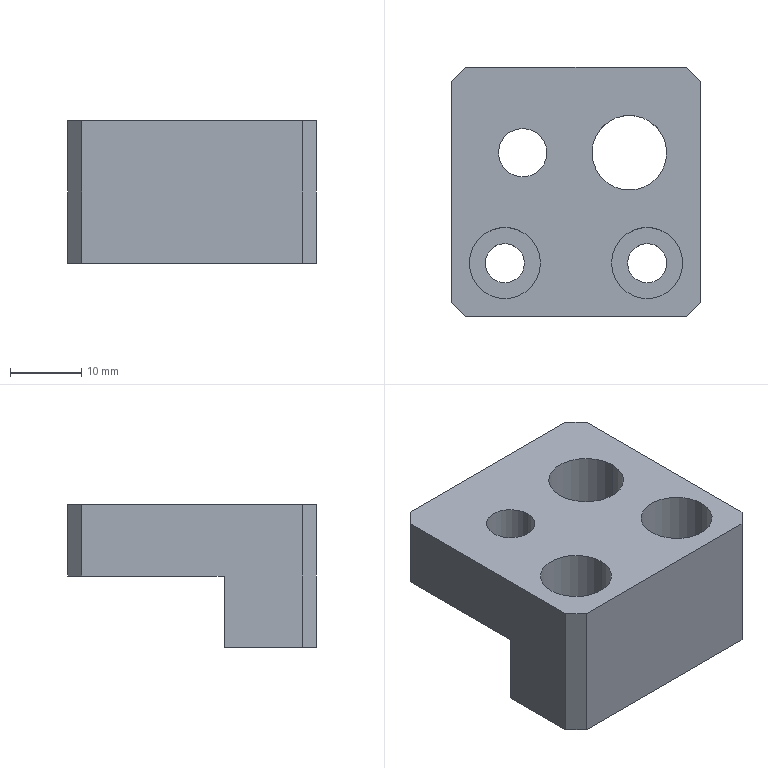Part | SolidWorks | features HoleWzd 3, Chamfer 1, Extrusion 1, ICE 1 | 1 solid | 26 faces | box 35 x 35 x 20 mm | volume 13186 mm3 | plane 14 | cylinder 12 | commonest cylinder face diameters 5.5 x4 10 x4 6.8 x2 10.5 x2
STEP:
#1=CARTESIAN_POINT('',(-15.,-10.,8.));
#2=VERTEX_POINT('',#1);
#3=CARTESIAN_POINT('',(-5.,-10.,8.));
#4=VERTEX_POINT('',#3);
#5=CARTESIAN_POINT('',(-10.,-10.,8.));
#6=DIRECTION('',(0.,0.,1.));
#7=DIRECTION('',(1.,0.,0.));
#8=AXIS2_PLACEMENT_3D('',#5,#6,#7);
#9=CIRCLE('',#8,5.);
#10=EDGE_CURVE('',#2,#4,#9,.T.);
#11=ORIENTED_EDGE('',*,*,#10,.F.);
#12=CARTESIAN_POINT('',(-15.,-10.,20.));
#13=VERTEX_POINT('',#12);
#14=CARTESIAN_POINT('',(-15.,-10.,20.));
#15=DIRECTION('',(0.,0.,1.));
#16=VECTOR('',#15,1000.);
#17=LINE('',#14,#16);
#18=EDGE_CURVE('',#2,#13,#17,.T.);
#19=ORIENTED_EDGE('',*,*,#18,.T.);
#20=CARTESIAN_POINT('',(-5.,-10.,20.));
#21=VERTEX_POINT('',#20);
#22=CARTESIAN_POINT('',(-10.,-10.,20.));
#23=DIRECTION('',(0.,0.,1.));
#24=DIRECTION('',(1.,0.,0.));
#25=AXIS2_PLACEMENT_3D('',#22,#23,#24);
#26=CIRCLE('',#25,5.);
#27=EDGE_CURVE('',#13,#21,#26,.T.);
#28=ORIENTED_EDGE('',*,*,#27,.T.);
#29=CARTESIAN_POINT('',(-5.,-10.,20.));
#30=DIRECTION('',(0.,0.,1.));
#31=VECTOR('',#30,1000.);
#32=LINE('',#29,#31);
#33=EDGE_CURVE('',#4,#21,#32,.T.);
#34=ORIENTED_EDGE('',*,*,#33,.F.);
#35=EDGE_LOOP('',(#11,#19,#28,#34));
#36=FACE_OUTER_BOUND('',#35,.T.);
#37=CARTESIAN_POINT('',(-10.,-10.,20.));
#38=DIRECTION('',(0.,0.,1.));
#39=DIRECTION('',(1.,0.,0.));
#40=AXIS2_PLACEMENT_3D('',#37,#38,#39);
#41=CYLINDRICAL_SURFACE('',#40,5.);
#42=ADVANCED_FACE('',(#36),#41,.F.);
#43=CARTESIAN_POINT('',(-12.75,-10.,0.));
#44=VERTEX_POINT('',#43);
#45=CARTESIAN_POINT('',(-7.25,-10.,0.));
#46=VERTEX_POINT('',#45);
#47=CARTESIAN_POINT('',(-10.,-10.,0.));
#48=DIRECTION('',(0.,0.,1.));
#49=DIRECTION('',(1.,0.,0.));
#50=AXIS2_PLACEMENT_3D('',#47,#48,#49);
#51=CIRCLE('',#50,2.75);
#52=EDGE_CURVE('',#44,#46,#51,.T.);
#53=ORIENTED_EDGE('',*,*,#52,.F.);
#54=CARTESIAN_POINT('',(-12.75,-10.,8.));
#55=VERTEX_POINT('',#54);
#56=CARTESIAN_POINT('',(-12.75,-10.,20.));
#57=DIRECTION('',(0.,0.,1.));
#58=VECTOR('',#57,1000.);
#59=LINE('',#56,#58);
#60=EDGE_CURVE('',#44,#55,#59,.T.);
#61=ORIENTED_EDGE('',*,*,#60,.T.);
#62=CARTESIAN_POINT('',(-7.25,-10.,8.));
#63=VERTEX_POINT('',#62);
#64=CARTESIAN_POINT('',(-10.,-10.,8.));
#65=DIRECTION('',(0.,0.,1.));
#66=DIRECTION('',(1.,0.,0.));
#67=AXIS2_PLACEMENT_3D('',#64,#65,#66);
#68=CIRCLE('',#67,2.75);
#69=EDGE_CURVE('',#55,#63,#68,.T.);
#70=ORIENTED_EDGE('',*,*,#69,.T.);
#71=CARTESIAN_POINT('',(-7.25,-10.,20.));
#72=DIRECTION('',(0.,0.,1.));
#73=VECTOR('',#72,1000.);
#74=LINE('',#71,#73);
#75=EDGE_CURVE('',#46,#63,#74,.T.);
#76=ORIENTED_EDGE('',*,*,#75,.F.);
#77=EDGE_LOOP('',(#53,#61,#70,#76));
#78=FACE_OUTER_BOUND('',#77,.T.);
#79=CARTESIAN_POINT('',(-10.,-10.,20.));
#80=DIRECTION('',(0.,0.,1.));
#81=DIRECTION('',(1.,0.,0.));
#82=AXIS2_PLACEMENT_3D('',#79,#80,#81);
#83=CYLINDRICAL_SURFACE('',#82,2.75);
#84=ADVANCED_FACE('',(#78),#83,.F.);
#85=CARTESIAN_POINT('',(5.,-10.,8.));
#86=VERTEX_POINT('',#85);
#87=CARTESIAN_POINT('',(15.,-10.,8.));
#88=VERTEX_POINT('',#87);
#89=CARTESIAN_POINT('',(10.,-10.,8.));
#90=DIRECTION('',(0.,0.,1.));
#91=DIRECTION('',(1.,0.,0.));
#92=AXIS2_PLACEMENT_3D('',#89,#90,#91);
#93=CIRCLE('',#92,5.);
#94=EDGE_CURVE('',#86,#88,#93,.T.);
#95=ORIENTED_EDGE('',*,*,#94,.F.);
#96=CARTESIAN_POINT('',(5.,-10.,20.));
#97=VERTEX_POINT('',#96);
#98=CARTESIAN_POINT('',(5.,-10.,20.));
#99=DIRECTION('',(0.,0.,1.));
#100=VECTOR('',#99,1000.);
#101=LINE('',#98,#100);
#102=EDGE_CURVE('',#86,#97,#101,.T.);
#103=ORIENTED_EDGE('',*,*,#102,.T.);
#104=CARTESIAN_POINT('',(15.,-10.,20.));
#105=VERTEX_POINT('',#104);
#106=CARTESIAN_POINT('',(10.,-10.,20.));
#107=DIRECTION('',(0.,0.,1.));
#108=DIRECTION('',(1.,0.,0.));
#109=AXIS2_PLACEMENT_3D('',#106,#107,#108);
#110=CIRCLE('',#109,5.);
#111=EDGE_CURVE('',#97,#105,#110,.T.);
#112=ORIENTED_EDGE('',*,*,#111,.T.);
#113=CARTESIAN_POINT('',(15.,-10.,20.));
#114=DIRECTION('',(0.,0.,1.));
#115=VECTOR('',#114,1000.);
#116=LINE('',#113,#115);
#117=EDGE_CURVE('',#88,#105,#116,.T.);
#118=ORIENTED_EDGE('',*,*,#117,.F.);
#119=EDGE_LOOP('',(#95,#103,#112,#118));
#120=FACE_OUTER_BOUND('',#119,.T.);
#121=CARTESIAN_POINT('',(10.,-10.,20.));
#122=DIRECTION('',(0.,0.,1.));
#123=DIRECTION('',(1.,0.,0.));
#124=AXIS2_PLACEMENT_3D('',#121,#122,#123);
#125=CYLINDRICAL_SURFACE('',#124,5.);
#126=ADVANCED_FACE('',(#120),#125,.F.);
#127=CARTESIAN_POINT('',(7.25,-10.,0.));
#128=VERTEX_POINT('',#127);
#129=CARTESIAN_POINT('',(12.75,-10.,0.));
#130=VERTEX_POINT('',#129);
#131=CARTESIAN_POINT('',(10.,-10.,0.));
#132=DIRECTION('',(0.,0.,1.));
#133=DIRECTION('',(1.,0.,0.));
#134=AXIS2_PLACEMENT_3D('',#131,#132,#133);
#135=CIRCLE('',#134,2.75);
#136=EDGE_CURVE('',#128,#130,#135,.T.);
#137=ORIENTED_EDGE('',*,*,#136,.F.);
#138=CARTESIAN_POINT('',(7.25,-10.,8.));
#139=VERTEX_POINT('',#138);
#140=CARTESIAN_POINT('',(7.25,-10.,20.));
#141=DIRECTION('',(0.,0.,1.));
#142=VECTOR('',#141,1000.);
#143=LINE('',#140,#142);
#144=EDGE_CURVE('',#128,#139,#143,.T.);
#145=ORIENTED_EDGE('',*,*,#144,.T.);
#146=CARTESIAN_POINT('',(12.75,-10.,8.));
#147=VERTEX_POINT('',#146);
#148=CARTESIAN_POINT('',(10.,-10.,8.));
#149=DIRECTION('',(0.,0.,1.));
#150=DIRECTION('',(1.,0.,0.));
#151=AXIS2_PLACEMENT_3D('',#148,#149,#150);
#152=CIRCLE('',#151,2.75);
#153=EDGE_CURVE('',#139,#147,#152,.T.);
#154=ORIENTED_EDGE('',*,*,#153,.T.);
#155=CARTESIAN_POINT('',(12.75,-10.,20.));
#156=DIRECTION('',(0.,0.,1.));
#157=VECTOR('',#156,1000.);
#158=LINE('',#155,#157);
#159=EDGE_CURVE('',#130,#147,#158,.T.);
#160=ORIENTED_EDGE('',*,*,#159,.F.);
#161=EDGE_LOOP('',(#137,#145,#154,#160));
#162=FACE_OUTER_BOUND('',#161,.T.);
#163=CARTESIAN_POINT('',(10.,-10.,20.));
#164=DIRECTION('',(0.,0.,1.));
#165=DIRECTION('',(1.,0.,0.));
#166=AXIS2_PLACEMENT_3D('',#163,#164,#165);
#167=CYLINDRICAL_SURFACE('',#166,2.75);
#168=ADVANCED_FACE('',(#162),#167,.F.);
#169=CARTESIAN_POINT('',(-4.1,5.5,10.));
#170=VERTEX_POINT('',#169);
#171=CARTESIAN_POINT('',(-10.9,5.5,10.));
#172=VERTEX_POINT('',#171);
#173=CARTESIAN_POINT('',(-7.5,5.5,10.));
#174=DIRECTION('',(0.,0.,-1.));
#175=DIRECTION('',(0.,-1.,0.));
#176=AXIS2_PLACEMENT_3D('',#173,#174,#175);
#177=CIRCLE('',#176,3.4);
#178=EDGE_CURVE('',#170,#172,#177,.T.);
#179=ORIENTED_EDGE('',*,*,#178,.T.);
#180=CARTESIAN_POINT('',(-10.9,5.5,20.));
#181=VERTEX_POINT('',#180);
#182=CARTESIAN_POINT('',(-10.9,5.5,20.));
#183=DIRECTION('',(0.,0.,1.));
#184=VECTOR('',#183,1000.);
#185=LINE('',#182,#184);
#186=EDGE_CURVE('',#172,#181,#185,.T.);
#187=ORIENTED_EDGE('',*,*,#186,.T.);
#188=CARTESIAN_POINT('',(-4.1,5.5,20.));
#189=VERTEX_POINT('',#188);
#190=CARTESIAN_POINT('',(-7.5,5.5,20.));
#191=DIRECTION('',(0.,0.,1.));
#192=DIRECTION('',(1.,0.,0.));
#193=AXIS2_PLACEMENT_3D('',#190,#191,#192);
#194=CIRCLE('',#193,3.4);
#195=EDGE_CURVE('',#181,#189,#194,.T.);
#196=ORIENTED_EDGE('',*,*,#195,.T.);
#197=CARTESIAN_POINT('',(-4.1,5.5,20.));
#198=DIRECTION('',(0.,0.,1.));
#199=VECTOR('',#198,1000.);
#200=LINE('',#197,#199);
#201=EDGE_CURVE('',#170,#189,#200,.T.);
#202=ORIENTED_EDGE('',*,*,#201,.F.);
#203=EDGE_LOOP('',(#179,#187,#196,#202));
#204=FACE_OUTER_BOUND('',#203,.T.);
#205=CARTESIAN_POINT('',(-7.5,5.5,20.));
#206=DIRECTION('',(0.,0.,1.));
#207=DIRECTION('',(1.,0.,0.));
#208=AXIS2_PLACEMENT_3D('',#205,#206,#207);
#209=CYLINDRICAL_SURFACE('',#208,3.4);
#210=ADVANCED_FACE('',(#204),#209,.F.);
#211=CARTESIAN_POINT('',(12.75,5.5,10.));
#212=VERTEX_POINT('',#211);
#213=CARTESIAN_POINT('',(2.25,5.5,10.));
#214=VERTEX_POINT('',#213);
#215=CARTESIAN_POINT('',(7.5,5.5,10.));
#216=DIRECTION('',(0.,0.,-1.));
#217=DIRECTION('',(0.,-1.,0.));
#218=AXIS2_PLACEMENT_3D('',#215,#216,#217);
#219=CIRCLE('',#218,5.25);
#220=EDGE_CURVE('',#212,#214,#219,.T.);
#221=ORIENTED_EDGE('',*,*,#220,.T.);
#222=CARTESIAN_POINT('',(2.25,5.5,20.));
#223=VERTEX_POINT('',#222);
#224=CARTESIAN_POINT('',(2.25,5.5,20.));
#225=DIRECTION('',(0.,0.,1.));
#226=VECTOR('',#225,1000.);
#227=LINE('',#224,#226);
#228=EDGE_CURVE('',#214,#223,#227,.T.);
#229=ORIENTED_EDGE('',*,*,#228,.T.);
#230=CARTESIAN_POINT('',(12.75,5.5,20.));
#231=VERTEX_POINT('',#230);
#232=CARTESIAN_POINT('',(7.5,5.5,20.));
#233=DIRECTION('',(0.,0.,1.));
#234=DIRECTION('',(1.,0.,0.));
#235=AXIS2_PLACEMENT_3D('',#232,#233,#234);
#236=CIRCLE('',#235,5.25);
#237=EDGE_CURVE('',#223,#231,#236,.T.);
#238=ORIENTED_EDGE('',*,*,#237,.T.);
#239=CARTESIAN_POINT('',(12.75,5.5,20.));
#240=DIRECTION('',(0.,0.,1.));
#241=VECTOR('',#240,1000.);
#242=LINE('',#239,#241);
#243=EDGE_CURVE('',#212,#231,#242,.T.);
#244=ORIENTED_EDGE('',*,*,#243,.F.);
#245=EDGE_LOOP('',(#221,#229,#238,#244));
#246=FACE_OUTER_BOUND('',#245,.T.);
#247=CARTESIAN_POINT('',(7.5,5.5,20.));
#248=DIRECTION('',(0.,0.,1.));
#249=DIRECTION('',(1.,0.,0.));
#250=AXIS2_PLACEMENT_3D('',#247,#248,#249);
#251=CYLINDRICAL_SURFACE('',#250,5.25);
#252=ADVANCED_FACE('',(#246),#251,.F.);
#253=CARTESIAN_POINT('',(17.5,-15.5,0.));
#254=VERTEX_POINT('',#253);
#255=CARTESIAN_POINT('',(17.5,-4.5,0.));
#256=VERTEX_POINT('',#255);
#257=CARTESIAN_POINT('',(17.5,-17.5,0.));
#258=DIRECTION('',(0.,1.,0.));
#259=VECTOR('',#258,1000.);
#260=LINE('',#257,#259);
#261=EDGE_CURVE('',#254,#256,#260,.T.);
#262=ORIENTED_EDGE('',*,*,#261,.T.);
#263=CARTESIAN_POINT('',(17.5,-4.5,10.));
#264=VERTEX_POINT('',#263);
#265=CARTESIAN_POINT('',(17.5,-4.5,0.));
#266=DIRECTION('',(0.,0.,-1.));
#267=VECTOR('',#266,1000.);
#268=LINE('',#265,#267);
#269=EDGE_CURVE('',#264,#256,#268,.T.);
#270=ORIENTED_EDGE('',*,*,#269,.F.);
#271=CARTESIAN_POINT('',(17.5,15.5,10.));
#272=VERTEX_POINT('',#271);
#273=CARTESIAN_POINT('',(17.5,17.5,10.));
#274=DIRECTION('',(0.,-1.,0.));
#275=VECTOR('',#274,1000.);
#276=LINE('',#273,#275);
#277=EDGE_CURVE('',#272,#264,#276,.T.);
#278=ORIENTED_EDGE('',*,*,#277,.F.);
#279=CARTESIAN_POINT('',(17.5,15.5,20.));
#280=VERTEX_POINT('',#279);
#281=CARTESIAN_POINT('',(17.5,15.5,20.));
#282=DIRECTION('',(0.,0.,1.));
#283=VECTOR('',#282,1000.);
#284=LINE('',#281,#283);
#285=EDGE_CURVE('',#272,#280,#284,.T.);
#286=ORIENTED_EDGE('',*,*,#285,.T.);
#287=CARTESIAN_POINT('',(17.5,-15.5,20.));
#288=VERTEX_POINT('',#287);
#289=CARTESIAN_POINT('',(17.5,-17.5,20.));
#290=DIRECTION('',(0.,1.,0.));
#291=VECTOR('',#290,1000.);
#292=LINE('',#289,#291);
#293=EDGE_CURVE('',#288,#280,#292,.T.);
#294=ORIENTED_EDGE('',*,*,#293,.F.);
#295=CARTESIAN_POINT('',(17.5,-15.5,20.));
#296=DIRECTION('',(0.,0.,-1.));
#297=VECTOR('',#296,1000.);
#298=LINE('',#295,#297);
#299=EDGE_CURVE('',#288,#254,#298,.T.);
#300=ORIENTED_EDGE('',*,*,#299,.T.);
#301=EDGE_LOOP('',(#262,#270,#278,#286,#294,#300));
#302=FACE_OUTER_BOUND('',#301,.T.);
#303=CARTESIAN_POINT('',(17.5,-17.5,20.));
#304=DIRECTION('',(-1.,0.,0.));
#305=DIRECTION('',(0.,0.,1.));
#306=AXIS2_PLACEMENT_3D('',#303,#304,#305);
#307=PLANE('',#306);
#308=ADVANCED_FACE('',(#302),#307,.F.);
#309=CARTESIAN_POINT('',(15.5,17.5,20.));
#310=VERTEX_POINT('',#309);
#311=CARTESIAN_POINT('',(15.5,17.5,10.));
#312=VERTEX_POINT('',#311);
#313=CARTESIAN_POINT('',(15.5,17.5,20.));
#314=DIRECTION('',(0.,0.,-1.));
#315=VECTOR('',#314,1000.);
#316=LINE('',#313,#315);
#317=EDGE_CURVE('',#310,#312,#316,.T.);
#318=ORIENTED_EDGE('',*,*,#317,.T.);
#319=CARTESIAN_POINT('',(-15.5,17.5,10.));
#320=VERTEX_POINT('',#319);
#321=CARTESIAN_POINT('',(-17.5,17.5,10.));
#322=DIRECTION('',(1.,0.,0.));
#323=VECTOR('',#322,1000.);
#324=LINE('',#321,#323);
#325=EDGE_CURVE('',#320,#312,#324,.T.);
#326=ORIENTED_EDGE('',*,*,#325,.F.);
#327=CARTESIAN_POINT('',(-15.5,17.5,20.));
#328=VERTEX_POINT('',#327);
#329=CARTESIAN_POINT('',(-15.5,17.5,20.));
#330=DIRECTION('',(0.,0.,1.));
#331=VECTOR('',#330,1000.);
#332=LINE('',#329,#331);
#333=EDGE_CURVE('',#320,#328,#332,.T.);
#334=ORIENTED_EDGE('',*,*,#333,.T.);
#335=CARTESIAN_POINT('',(-17.5,17.5,20.));
#336=DIRECTION('',(-1.,0.,0.));
#337=VECTOR('',#336,1000.);
#338=LINE('',#335,#337);
#339=EDGE_CURVE('',#310,#328,#338,.T.);
#340=ORIENTED_EDGE('',*,*,#339,.F.);
#341=EDGE_LOOP('',(#318,#326,#334,#340));
#342=FACE_OUTER_BOUND('',#341,.T.);
#343=CARTESIAN_POINT('',(-17.5,17.5,20.));
#344=DIRECTION('',(0.,-1.,0.));
#345=DIRECTION('',(0.,0.,-1.));
#346=AXIS2_PLACEMENT_3D('',#343,#344,#345);
#347=PLANE('',#346);
#348=ADVANCED_FACE('',(#342),#347,.F.);
#349=CARTESIAN_POINT('',(-17.5,15.5,10.));
#350=VERTEX_POINT('',#349);
#351=CARTESIAN_POINT('',(-17.5,-4.5,10.));
#352=VERTEX_POINT('',#351);
#353=CARTESIAN_POINT('',(-17.5,17.5,10.));
#354=DIRECTION('',(0.,-1.,0.));
#355=VECTOR('',#354,1000.);
#356=LINE('',#353,#355);
#357=EDGE_CURVE('',#350,#352,#356,.T.);
#358=ORIENTED_EDGE('',*,*,#357,.T.);
#359=CARTESIAN_POINT('',(-17.5,-4.5,0.));
#360=VERTEX_POINT('',#359);
#361=CARTESIAN_POINT('',(-17.5,-4.5,0.));
#362=DIRECTION('',(0.,0.,-1.));
#363=VECTOR('',#362,1000.);
#364=LINE('',#361,#363);
#365=EDGE_CURVE('',#352,#360,#364,.T.);
#366=ORIENTED_EDGE('',*,*,#365,.T.);
#367=CARTESIAN_POINT('',(-17.5,-15.5,0.));
#368=VERTEX_POINT('',#367);
#369=CARTESIAN_POINT('',(-17.5,-17.5,0.));
#370=DIRECTION('',(0.,-1.,0.));
#371=VECTOR('',#370,1000.);
#372=LINE('',#369,#371);
#373=EDGE_CURVE('',#360,#368,#372,.T.);
#374=ORIENTED_EDGE('',*,*,#373,.T.);
#375=CARTESIAN_POINT('',(-17.5,-15.5,20.));
#376=VERTEX_POINT('',#375);
#377=CARTESIAN_POINT('',(-17.5,-15.5,20.));
#378=DIRECTION('',(0.,0.,1.));
#379=VECTOR('',#378,1000.);
#380=LINE('',#377,#379);
#381=EDGE_CURVE('',#368,#376,#380,.T.);
#382=ORIENTED_EDGE('',*,*,#381,.T.);
#383=CARTESIAN_POINT('',(-17.5,15.5,20.));
#384=VERTEX_POINT('',#383);
#385=CARTESIAN_POINT('',(-17.5,-17.5,20.));
#386=DIRECTION('',(0.,-1.,0.));
#387=VECTOR('',#386,1000.);
#388=LINE('',#385,#387);
#389=EDGE_CURVE('',#384,#376,#388,.T.);
#390=ORIENTED_EDGE('',*,*,#389,.F.);
#391=CARTESIAN_POINT('',(-17.5,15.5,20.));
#392=DIRECTION('',(0.,0.,-1.));
#393=VECTOR('',#392,1000.);
#394=LINE('',#391,#393);
#395=EDGE_CURVE('',#384,#350,#394,.T.);
#396=ORIENTED_EDGE('',*,*,#395,.T.);
#397=EDGE_LOOP('',(#358,#366,#374,#382,#390,#396));
#398=FACE_OUTER_BOUND('',#397,.T.);
#399=CARTESIAN_POINT('',(-17.5,-17.5,20.));
#400=DIRECTION('',(1.,0.,0.));
#401=DIRECTION('',(0.,0.,-1.));
#402=AXIS2_PLACEMENT_3D('',#399,#400,#401);
#403=PLANE('',#402);
#404=ADVANCED_FACE('',(#398),#403,.F.);
#405=CARTESIAN_POINT('',(-15.5,-17.5,0.));
#406=VERTEX_POINT('',#405);
#407=CARTESIAN_POINT('',(15.5,-17.5,0.));
#408=VERTEX_POINT('',#407);
#409=CARTESIAN_POINT('',(-17.5,-17.5,0.));
#410=DIRECTION('',(1.,0.,0.));
#411=VECTOR('',#410,1000.);
#412=LINE('',#409,#411);
#413=EDGE_CURVE('',#406,#408,#412,.T.);
#414=ORIENTED_EDGE('',*,*,#413,.T.);
#415=CARTESIAN_POINT('',(15.5,-17.5,20.));
#416=VERTEX_POINT('',#415);
#417=CARTESIAN_POINT('',(15.5,-17.5,20.));
#418=DIRECTION('',(0.,0.,1.));
#419=VECTOR('',#418,1000.);
#420=LINE('',#417,#419);
#421=EDGE_CURVE('',#408,#416,#420,.T.);
#422=ORIENTED_EDGE('',*,*,#421,.T.);
#423=CARTESIAN_POINT('',(-15.5,-17.5,20.));
#424=VERTEX_POINT('',#423);
#425=CARTESIAN_POINT('',(-17.5,-17.5,20.));
#426=DIRECTION('',(1.,0.,0.));
#427=VECTOR('',#426,1000.);
#428=LINE('',#425,#427);
#429=EDGE_CURVE('',#424,#416,#428,.T.);
#430=ORIENTED_EDGE('',*,*,#429,.F.);
#431=CARTESIAN_POINT('',(-15.5,-17.5,20.));
#432=DIRECTION('',(0.,0.,-1.));
#433=VECTOR('',#432,1000.);
#434=LINE('',#431,#433);
#435=EDGE_CURVE('',#424,#406,#434,.T.);
#436=ORIENTED_EDGE('',*,*,#435,.T.);
#437=EDGE_LOOP('',(#414,#422,#430,#436));
#438=FACE_OUTER_BOUND('',#437,.T.);
#439=CARTESIAN_POINT('',(-17.5,-17.5,20.));
#440=DIRECTION('',(0.,1.,0.));
#441=DIRECTION('',(0.,0.,1.));
#442=AXIS2_PLACEMENT_3D('',#439,#440,#441);
#443=PLANE('',#442);
#444=ADVANCED_FACE('',(#438),#443,.F.);
#445=CARTESIAN_POINT('',(-10.,-10.,20.));
#446=DIRECTION('',(0.,0.,1.));
#447=DIRECTION('',(1.,0.,0.));
#448=AXIS2_PLACEMENT_3D('',#445,#446,#447);
#449=CIRCLE('',#448,5.);
#450=EDGE_CURVE('',#21,#13,#449,.T.);
#451=ORIENTED_EDGE('',*,*,#450,.F.);
#452=ORIENTED_EDGE('',*,*,#27,.F.);
#453=EDGE_LOOP('',(#451,#452));
#454=FACE_BOUND('',#453,.T.);
#455=CARTESIAN_POINT('',(10.,-10.,20.));
#456=DIRECTION('',(0.,0.,1.));
#457=DIRECTION('',(1.,0.,0.));
#458=AXIS2_PLACEMENT_3D('',#455,#456,#457);
#459=CIRCLE('',#458,5.);
#460=EDGE_CURVE('',#105,#97,#459,.T.);
#461=ORIENTED_EDGE('',*,*,#460,.F.);
#462=ORIENTED_EDGE('',*,*,#111,.F.);
#463=EDGE_LOOP('',(#461,#462));
#464=FACE_BOUND('',#463,.T.);
#465=CARTESIAN_POINT('',(-7.5,5.5,20.));
#466=DIRECTION('',(0.,0.,1.));
#467=DIRECTION('',(1.,0.,0.));
#468=AXIS2_PLACEMENT_3D('',#465,#466,#467);
#469=CIRCLE('',#468,3.4);
#470=EDGE_CURVE('',#189,#181,#469,.T.);
#471=ORIENTED_EDGE('',*,*,#470,.F.);
#472=ORIENTED_EDGE('',*,*,#195,.F.);
#473=EDGE_LOOP('',(#471,#472));
#474=FACE_BOUND('',#473,.T.);
#475=CARTESIAN_POINT('',(7.5,5.5,20.));
#476=DIRECTION('',(0.,0.,1.));
#477=DIRECTION('',(1.,0.,0.));
#478=AXIS2_PLACEMENT_3D('',#475,#476,#477);
#479=CIRCLE('',#478,5.25);
#480=EDGE_CURVE('',#231,#223,#479,.T.);
#481=ORIENTED_EDGE('',*,*,#480,.F.);
#482=ORIENTED_EDGE('',*,*,#237,.F.);
#483=EDGE_LOOP('',(#481,#482));
#484=FACE_BOUND('',#483,.T.);
#485=ORIENTED_EDGE('',*,*,#429,.T.);
#486=CARTESIAN_POINT('',(17.5,-15.5,20.));
#487=DIRECTION('',(0.7071,0.7071,0.));
#488=VECTOR('',#487,1000.);
#489=LINE('',#486,#488);
#490=EDGE_CURVE('',#416,#288,#489,.T.);
#491=ORIENTED_EDGE('',*,*,#490,.T.);
#492=ORIENTED_EDGE('',*,*,#293,.T.);
#493=CARTESIAN_POINT('',(15.5,17.5,20.));
#494=DIRECTION('',(-0.7071,0.7071,0.));
#495=VECTOR('',#494,1000.);
#496=LINE('',#493,#495);
#497=EDGE_CURVE('',#280,#310,#496,.T.);
#498=ORIENTED_EDGE('',*,*,#497,.T.);
#499=ORIENTED_EDGE('',*,*,#339,.T.);
#500=CARTESIAN_POINT('',(-17.5,15.5,20.));
#501=DIRECTION('',(-0.7071,-0.7071,0.));
#502=VECTOR('',#501,1000.);
#503=LINE('',#500,#502);
#504=EDGE_CURVE('',#328,#384,#503,.T.);
#505=ORIENTED_EDGE('',*,*,#504,.T.);
#506=ORIENTED_EDGE('',*,*,#389,.T.);
#507=CARTESIAN_POINT('',(-15.5,-17.5,20.));
#508=DIRECTION('',(0.7071,-0.7071,0.));
#509=VECTOR('',#508,1000.);
#510=LINE('',#507,#509);
#511=EDGE_CURVE('',#376,#424,#510,.T.);
#512=ORIENTED_EDGE('',*,*,#511,.T.);
#513=EDGE_LOOP('',(#485,#491,#492,#498,#499,#505,#506,#512));
#514=FACE_OUTER_BOUND('',#513,.T.);
#515=CARTESIAN_POINT('',(0.,0.,20.));
#516=DIRECTION('',(0.,0.,-1.));
#517=DIRECTION('',(-1.,0.,0.));
#518=AXIS2_PLACEMENT_3D('',#515,#516,#517);
#519=PLANE('',#518);
#520=ADVANCED_FACE('',(#454,#464,#474,#484,#514),#519,.F.);
#521=CARTESIAN_POINT('',(-17.5,-4.5,0.));
#522=DIRECTION('',(1.,0.,0.));
#523=VECTOR('',#522,1000.);
#524=LINE('',#521,#523);
#525=EDGE_CURVE('',#360,#256,#524,.T.);
#526=ORIENTED_EDGE('',*,*,#525,.T.);
#527=ORIENTED_EDGE('',*,*,#261,.F.);
#528=CARTESIAN_POINT('',(16.5,-16.5,0.));
#529=DIRECTION('',(-0.7071,-0.7071,0.));
#530=VECTOR('',#529,1000.);
#531=LINE('',#528,#530);
#532=EDGE_CURVE('',#254,#408,#531,.T.);
#533=ORIENTED_EDGE('',*,*,#532,.T.);
#534=ORIENTED_EDGE('',*,*,#413,.F.);
#535=CARTESIAN_POINT('',(-16.5,-16.5,0.));
#536=DIRECTION('',(-0.7071,0.7071,0.));
#537=VECTOR('',#536,1000.);
#538=LINE('',#535,#537);
#539=EDGE_CURVE('',#406,#368,#538,.T.);
#540=ORIENTED_EDGE('',*,*,#539,.T.);
#541=ORIENTED_EDGE('',*,*,#373,.F.);
#542=EDGE_LOOP('',(#526,#527,#533,#534,#540,#541));
#543=FACE_OUTER_BOUND('',#542,.T.);
#544=CARTESIAN_POINT('',(-10.,-10.,0.));
#545=DIRECTION('',(0.,0.,1.));
#546=DIRECTION('',(1.,0.,0.));
#547=AXIS2_PLACEMENT_3D('',#544,#545,#546);
#548=CIRCLE('',#547,2.75);
#549=EDGE_CURVE('',#46,#44,#548,.T.);
#550=ORIENTED_EDGE('',*,*,#549,.T.);
#551=ORIENTED_EDGE('',*,*,#52,.T.);
#552=EDGE_LOOP('',(#550,#551));
#553=FACE_BOUND('',#552,.T.);
#554=CARTESIAN_POINT('',(10.,-10.,0.));
#555=DIRECTION('',(0.,0.,1.));
#556=DIRECTION('',(1.,0.,0.));
#557=AXIS2_PLACEMENT_3D('',#554,#555,#556);
#558=CIRCLE('',#557,2.75);
#559=EDGE_CURVE('',#130,#128,#558,.T.);
#560=ORIENTED_EDGE('',*,*,#559,.T.);
#561=ORIENTED_EDGE('',*,*,#136,.T.);
#562=EDGE_LOOP('',(#560,#561));
#563=FACE_BOUND('',#562,.T.);
#564=CARTESIAN_POINT('',(0.,0.,0.));
#565=DIRECTION('',(0.,0.,-1.));
#566=DIRECTION('',(-1.,0.,0.));
#567=AXIS2_PLACEMENT_3D('',#564,#565,#566);
#568=PLANE('',#567);
#569=ADVANCED_FACE('',(#543,#553,#563),#568,.T.);
#570=ORIENTED_EDGE('',*,*,#490,.F.);
#571=ORIENTED_EDGE('',*,*,#421,.F.);
#572=ORIENTED_EDGE('',*,*,#532,.F.);
#573=ORIENTED_EDGE('',*,*,#299,.F.);
#574=EDGE_LOOP('',(#570,#571,#572,#573));
#575=FACE_OUTER_BOUND('',#574,.T.);
#576=CARTESIAN_POINT('',(17.5,-15.5,20.));
#577=DIRECTION('',(-0.7071,0.7071,0.));
#578=DIRECTION('',(0.,0.,-1.));
#579=AXIS2_PLACEMENT_3D('',#576,#577,#578);
#580=PLANE('',#579);
#581=ADVANCED_FACE('',(#575),#580,.F.);
#582=ORIENTED_EDGE('',*,*,#511,.F.);
#583=ORIENTED_EDGE('',*,*,#381,.F.);
#584=ORIENTED_EDGE('',*,*,#539,.F.);
#585=ORIENTED_EDGE('',*,*,#435,.F.);
#586=EDGE_LOOP('',(#582,#583,#584,#585));
#587=FACE_OUTER_BOUND('',#586,.T.);
#588=CARTESIAN_POINT('',(-15.5,-17.5,20.));
#589=DIRECTION('',(0.7071,0.7071,0.));
#590=DIRECTION('',(0.,0.,-1.));
#591=AXIS2_PLACEMENT_3D('',#588,#589,#590);
#592=PLANE('',#591);
#593=ADVANCED_FACE('',(#587),#592,.F.);
#594=CARTESIAN_POINT('',(-17.5,15.5,10.));
#595=DIRECTION('',(0.7071,0.7071,0.));
#596=VECTOR('',#595,1000.);
#597=LINE('',#594,#596);
#598=EDGE_CURVE('',#350,#320,#597,.T.);
#599=ORIENTED_EDGE('',*,*,#598,.F.);
#600=ORIENTED_EDGE('',*,*,#395,.F.);
#601=ORIENTED_EDGE('',*,*,#504,.F.);
#602=ORIENTED_EDGE('',*,*,#333,.F.);
#603=EDGE_LOOP('',(#599,#600,#601,#602));
#604=FACE_OUTER_BOUND('',#603,.T.);
#605=CARTESIAN_POINT('',(-17.5,15.5,20.));
#606=DIRECTION('',(0.7071,-0.7071,0.));
#607=DIRECTION('',(0.,0.,-1.));
#608=AXIS2_PLACEMENT_3D('',#605,#606,#607);
#609=PLANE('',#608);
#610=ADVANCED_FACE('',(#604),#609,.F.);
#611=CARTESIAN_POINT('',(15.5,17.5,10.));
#612=DIRECTION('',(0.7071,-0.7071,0.));
#613=VECTOR('',#612,1000.);
#614=LINE('',#611,#613);
#615=EDGE_CURVE('',#312,#272,#614,.T.);
#616=ORIENTED_EDGE('',*,*,#615,.F.);
#617=ORIENTED_EDGE('',*,*,#317,.F.);
#618=ORIENTED_EDGE('',*,*,#497,.F.);
#619=ORIENTED_EDGE('',*,*,#285,.F.);
#620=EDGE_LOOP('',(#616,#617,#618,#619));
#621=FACE_OUTER_BOUND('',#620,.T.);
#622=CARTESIAN_POINT('',(15.5,17.5,20.));
#623=DIRECTION('',(-0.7071,-0.7071,0.));
#624=DIRECTION('',(0.,0.,-1.));
#625=AXIS2_PLACEMENT_3D('',#622,#623,#624);
#626=PLANE('',#625);
#627=ADVANCED_FACE('',(#621),#626,.F.);
#628=ORIENTED_EDGE('',*,*,#228,.F.);
#629=CARTESIAN_POINT('',(7.5,5.5,10.));
#630=DIRECTION('',(0.,0.,-1.));
#631=DIRECTION('',(0.,-1.,0.));
#632=AXIS2_PLACEMENT_3D('',#629,#630,#631);
#633=CIRCLE('',#632,5.25);
#634=EDGE_CURVE('',#214,#212,#633,.T.);
#635=ORIENTED_EDGE('',*,*,#634,.T.);
#636=ORIENTED_EDGE('',*,*,#243,.T.);
#637=ORIENTED_EDGE('',*,*,#480,.T.);
#638=EDGE_LOOP('',(#628,#635,#636,#637));
#639=FACE_OUTER_BOUND('',#638,.T.);
#640=CARTESIAN_POINT('',(7.5,5.5,20.));
#641=DIRECTION('',(0.,0.,1.));
#642=DIRECTION('',(1.,0.,0.));
#643=AXIS2_PLACEMENT_3D('',#640,#641,#642);
#644=CYLINDRICAL_SURFACE('',#643,5.25);
#645=ADVANCED_FACE('',(#639),#644,.F.);
#646=ORIENTED_EDGE('',*,*,#186,.F.);
#647=CARTESIAN_POINT('',(-7.5,5.5,10.));
#648=DIRECTION('',(0.,0.,-1.));
#649=DIRECTION('',(0.,-1.,0.));
#650=AXIS2_PLACEMENT_3D('',#647,#648,#649);
#651=CIRCLE('',#650,3.4);
#652=EDGE_CURVE('',#172,#170,#651,.T.);
#653=ORIENTED_EDGE('',*,*,#652,.T.);
#654=ORIENTED_EDGE('',*,*,#201,.T.);
#655=ORIENTED_EDGE('',*,*,#470,.T.);
#656=EDGE_LOOP('',(#646,#653,#654,#655));
#657=FACE_OUTER_BOUND('',#656,.T.);
#658=CARTESIAN_POINT('',(-7.5,5.5,20.));
#659=DIRECTION('',(0.,0.,1.));
#660=DIRECTION('',(1.,0.,0.));
#661=AXIS2_PLACEMENT_3D('',#658,#659,#660);
#662=CYLINDRICAL_SURFACE('',#661,3.4);
#663=ADVANCED_FACE('',(#657),#662,.F.);
#664=ORIENTED_EDGE('',*,*,#144,.F.);
#665=ORIENTED_EDGE('',*,*,#559,.F.);
#666=ORIENTED_EDGE('',*,*,#159,.T.);
#667=CARTESIAN_POINT('',(10.,-10.,8.));
#668=DIRECTION('',(0.,0.,1.));
#669=DIRECTION('',(1.,0.,0.));
#670=AXIS2_PLACEMENT_3D('',#667,#668,#669);
#671=CIRCLE('',#670,2.75);
#672=EDGE_CURVE('',#147,#139,#671,.T.);
#673=ORIENTED_EDGE('',*,*,#672,.T.);
#674=EDGE_LOOP('',(#664,#665,#666,#673));
#675=FACE_OUTER_BOUND('',#674,.T.);
#676=CARTESIAN_POINT('',(10.,-10.,20.));
#677=DIRECTION('',(0.,0.,1.));
#678=DIRECTION('',(1.,0.,0.));
#679=AXIS2_PLACEMENT_3D('',#676,#677,#678);
#680=CYLINDRICAL_SURFACE('',#679,2.75);
#681=ADVANCED_FACE('',(#675),#680,.F.);
#682=ORIENTED_EDGE('',*,*,#672,.F.);
#683=ORIENTED_EDGE('',*,*,#153,.F.);
#684=EDGE_LOOP('',(#682,#683));
#685=FACE_BOUND('',#684,.T.);
#686=CARTESIAN_POINT('',(10.,-10.,8.));
#687=DIRECTION('',(0.,0.,1.));
#688=DIRECTION('',(1.,0.,0.));
#689=AXIS2_PLACEMENT_3D('',#686,#687,#688);
#690=CIRCLE('',#689,5.);
#691=EDGE_CURVE('',#88,#86,#690,.T.);
#692=ORIENTED_EDGE('',*,*,#691,.T.);
#693=ORIENTED_EDGE('',*,*,#94,.T.);
#694=EDGE_LOOP('',(#692,#693));
#695=FACE_OUTER_BOUND('',#694,.T.);
#696=CARTESIAN_POINT('',(12.75,-10.,8.));
#697=DIRECTION('',(0.,0.,-1.));
#698=DIRECTION('',(-1.,0.,0.));
#699=AXIS2_PLACEMENT_3D('',#696,#697,#698);
#700=PLANE('',#699);
#701=ADVANCED_FACE('',(#685,#695),#700,.F.);
#702=ORIENTED_EDGE('',*,*,#102,.F.);
#703=ORIENTED_EDGE('',*,*,#691,.F.);
#704=ORIENTED_EDGE('',*,*,#117,.T.);
#705=ORIENTED_EDGE('',*,*,#460,.T.);
#706=EDGE_LOOP('',(#702,#703,#704,#705));
#707=FACE_OUTER_BOUND('',#706,.T.);
#708=CARTESIAN_POINT('',(10.,-10.,20.));
#709=DIRECTION('',(0.,0.,1.));
#710=DIRECTION('',(1.,0.,0.));
#711=AXIS2_PLACEMENT_3D('',#708,#709,#710);
#712=CYLINDRICAL_SURFACE('',#711,5.);
#713=ADVANCED_FACE('',(#707),#712,.F.);
#714=ORIENTED_EDGE('',*,*,#60,.F.);
#715=ORIENTED_EDGE('',*,*,#549,.F.);
#716=ORIENTED_EDGE('',*,*,#75,.T.);
#717=CARTESIAN_POINT('',(-10.,-10.,8.));
#718=DIRECTION('',(0.,0.,1.));
#719=DIRECTION('',(1.,0.,0.));
#720=AXIS2_PLACEMENT_3D('',#717,#718,#719);
#721=CIRCLE('',#720,2.75);
#722=EDGE_CURVE('',#63,#55,#721,.T.);
#723=ORIENTED_EDGE('',*,*,#722,.T.);
#724=EDGE_LOOP('',(#714,#715,#716,#723));
#725=FACE_OUTER_BOUND('',#724,.T.);
#726=CARTESIAN_POINT('',(-10.,-10.,20.));
#727=DIRECTION('',(0.,0.,1.));
#728=DIRECTION('',(1.,0.,0.));
#729=AXIS2_PLACEMENT_3D('',#726,#727,#728);
#730=CYLINDRICAL_SURFACE('',#729,2.75);
#731=ADVANCED_FACE('',(#725),#730,.F.);
#732=ORIENTED_EDGE('',*,*,#722,.F.);
#733=ORIENTED_EDGE('',*,*,#69,.F.);
#734=EDGE_LOOP('',(#732,#733));
#735=FACE_BOUND('',#734,.T.);
#736=CARTESIAN_POINT('',(-10.,-10.,8.));
#737=DIRECTION('',(0.,0.,1.));
#738=DIRECTION('',(1.,0.,0.));
#739=AXIS2_PLACEMENT_3D('',#736,#737,#738);
#740=CIRCLE('',#739,5.);
#741=EDGE_CURVE('',#4,#2,#740,.T.);
#742=ORIENTED_EDGE('',*,*,#741,.T.);
#743=ORIENTED_EDGE('',*,*,#10,.T.);
#744=EDGE_LOOP('',(#742,#743));
#745=FACE_OUTER_BOUND('',#744,.T.);
#746=CARTESIAN_POINT('',(-7.25,-10.,8.));
#747=DIRECTION('',(0.,0.,-1.));
#748=DIRECTION('',(-1.,0.,0.));
#749=AXIS2_PLACEMENT_3D('',#746,#747,#748);
#750=PLANE('',#749);
#751=ADVANCED_FACE('',(#735,#745),#750,.F.);
#752=ORIENTED_EDGE('',*,*,#18,.F.);
#753=ORIENTED_EDGE('',*,*,#741,.F.);
#754=ORIENTED_EDGE('',*,*,#33,.T.);
#755=ORIENTED_EDGE('',*,*,#450,.T.);
#756=EDGE_LOOP('',(#752,#753,#754,#755));
#757=FACE_OUTER_BOUND('',#756,.T.);
#758=CARTESIAN_POINT('',(-10.,-10.,20.));
#759=DIRECTION('',(0.,0.,1.));
#760=DIRECTION('',(1.,0.,0.));
#761=AXIS2_PLACEMENT_3D('',#758,#759,#760);
#762=CYLINDRICAL_SURFACE('',#761,5.);
#763=ADVANCED_FACE('',(#757),#762,.F.);
#764=ORIENTED_EDGE('',*,*,#598,.T.);
#765=ORIENTED_EDGE('',*,*,#325,.T.);
#766=ORIENTED_EDGE('',*,*,#615,.T.);
#767=ORIENTED_EDGE('',*,*,#277,.T.);
#768=CARTESIAN_POINT('',(-17.5,-4.5,10.));
#769=DIRECTION('',(1.,0.,0.));
#770=VECTOR('',#769,1000.);
#771=LINE('',#768,#770);
#772=EDGE_CURVE('',#352,#264,#771,.T.);
#773=ORIENTED_EDGE('',*,*,#772,.F.);
#774=ORIENTED_EDGE('',*,*,#357,.F.);
#775=EDGE_LOOP('',(#764,#765,#766,#767,#773,#774));
#776=FACE_OUTER_BOUND('',#775,.T.);
#777=ORIENTED_EDGE('',*,*,#178,.F.);
#778=ORIENTED_EDGE('',*,*,#652,.F.);
#779=EDGE_LOOP('',(#777,#778));
#780=FACE_BOUND('',#779,.T.);
#781=ORIENTED_EDGE('',*,*,#220,.F.);
#782=ORIENTED_EDGE('',*,*,#634,.F.);
#783=EDGE_LOOP('',(#781,#782));
#784=FACE_BOUND('',#783,.T.);
#785=CARTESIAN_POINT('',(-17.5,17.5,10.));
#786=DIRECTION('',(0.,0.,1.));
#787=DIRECTION('',(0.,-1.,0.));
#788=AXIS2_PLACEMENT_3D('',#785,#786,#787);
#789=PLANE('',#788);
#790=ADVANCED_FACE('',(#776,#780,#784),#789,.F.);
#791=ORIENTED_EDGE('',*,*,#269,.T.);
#792=ORIENTED_EDGE('',*,*,#525,.F.);
#793=ORIENTED_EDGE('',*,*,#365,.F.);
#794=ORIENTED_EDGE('',*,*,#772,.T.);
#795=EDGE_LOOP('',(#791,#792,#793,#794));
#796=FACE_OUTER_BOUND('',#795,.T.);
#797=CARTESIAN_POINT('',(-17.5,-4.5,0.));
#798=DIRECTION('',(0.,-1.,0.));
#799=DIRECTION('',(0.,0.,-1.));
#800=AXIS2_PLACEMENT_3D('',#797,#798,#799);
#801=PLANE('',#800);
#802=ADVANCED_FACE('',(#796),#801,.F.);
#803=CLOSED_SHELL('',(#42,#84,#126,#168,#210,#252,#308,#348,#404,#444,#520,#569,#581,#593,#610,#627,#645,#663,#681,#701,#713,#731,#751,#763,#790,#802));
#804=MANIFOLD_SOLID_BREP('',#803);
#805=CARTESIAN_POINT('',(0.,0.,0.));
#806=DIRECTION('',(0.,0.,1.));
#807=DIRECTION('',(1.,0.,0.));
#808=AXIS2_PLACEMENT_3D('',#805,#806,#807);
#809=(LENGTH_UNIT()NAMED_UNIT(*)SI_UNIT(.MILLI.,.METRE.));
#810=UNCERTAINTY_MEASURE_WITH_UNIT(LENGTH_MEASURE(0.00001),#809,'','');
#811=(NAMED_UNIT(*)PLANE_ANGLE_UNIT()SI_UNIT($,.RADIAN.));
#812=(NAMED_UNIT(*)SI_UNIT($,.STERADIAN.)SOLID_ANGLE_UNIT());
#813=(GEOMETRIC_REPRESENTATION_CONTEXT(3)GLOBAL_UNCERTAINTY_ASSIGNED_CONTEXT((#810))GLOBAL_UNIT_ASSIGNED_CONTEXT((#809,#811,#812))REPRESENTATION_CONTEXT('',''));
#814=ADVANCED_BREP_SHAPE_REPRESENTATION('',(#804,#808),#813);